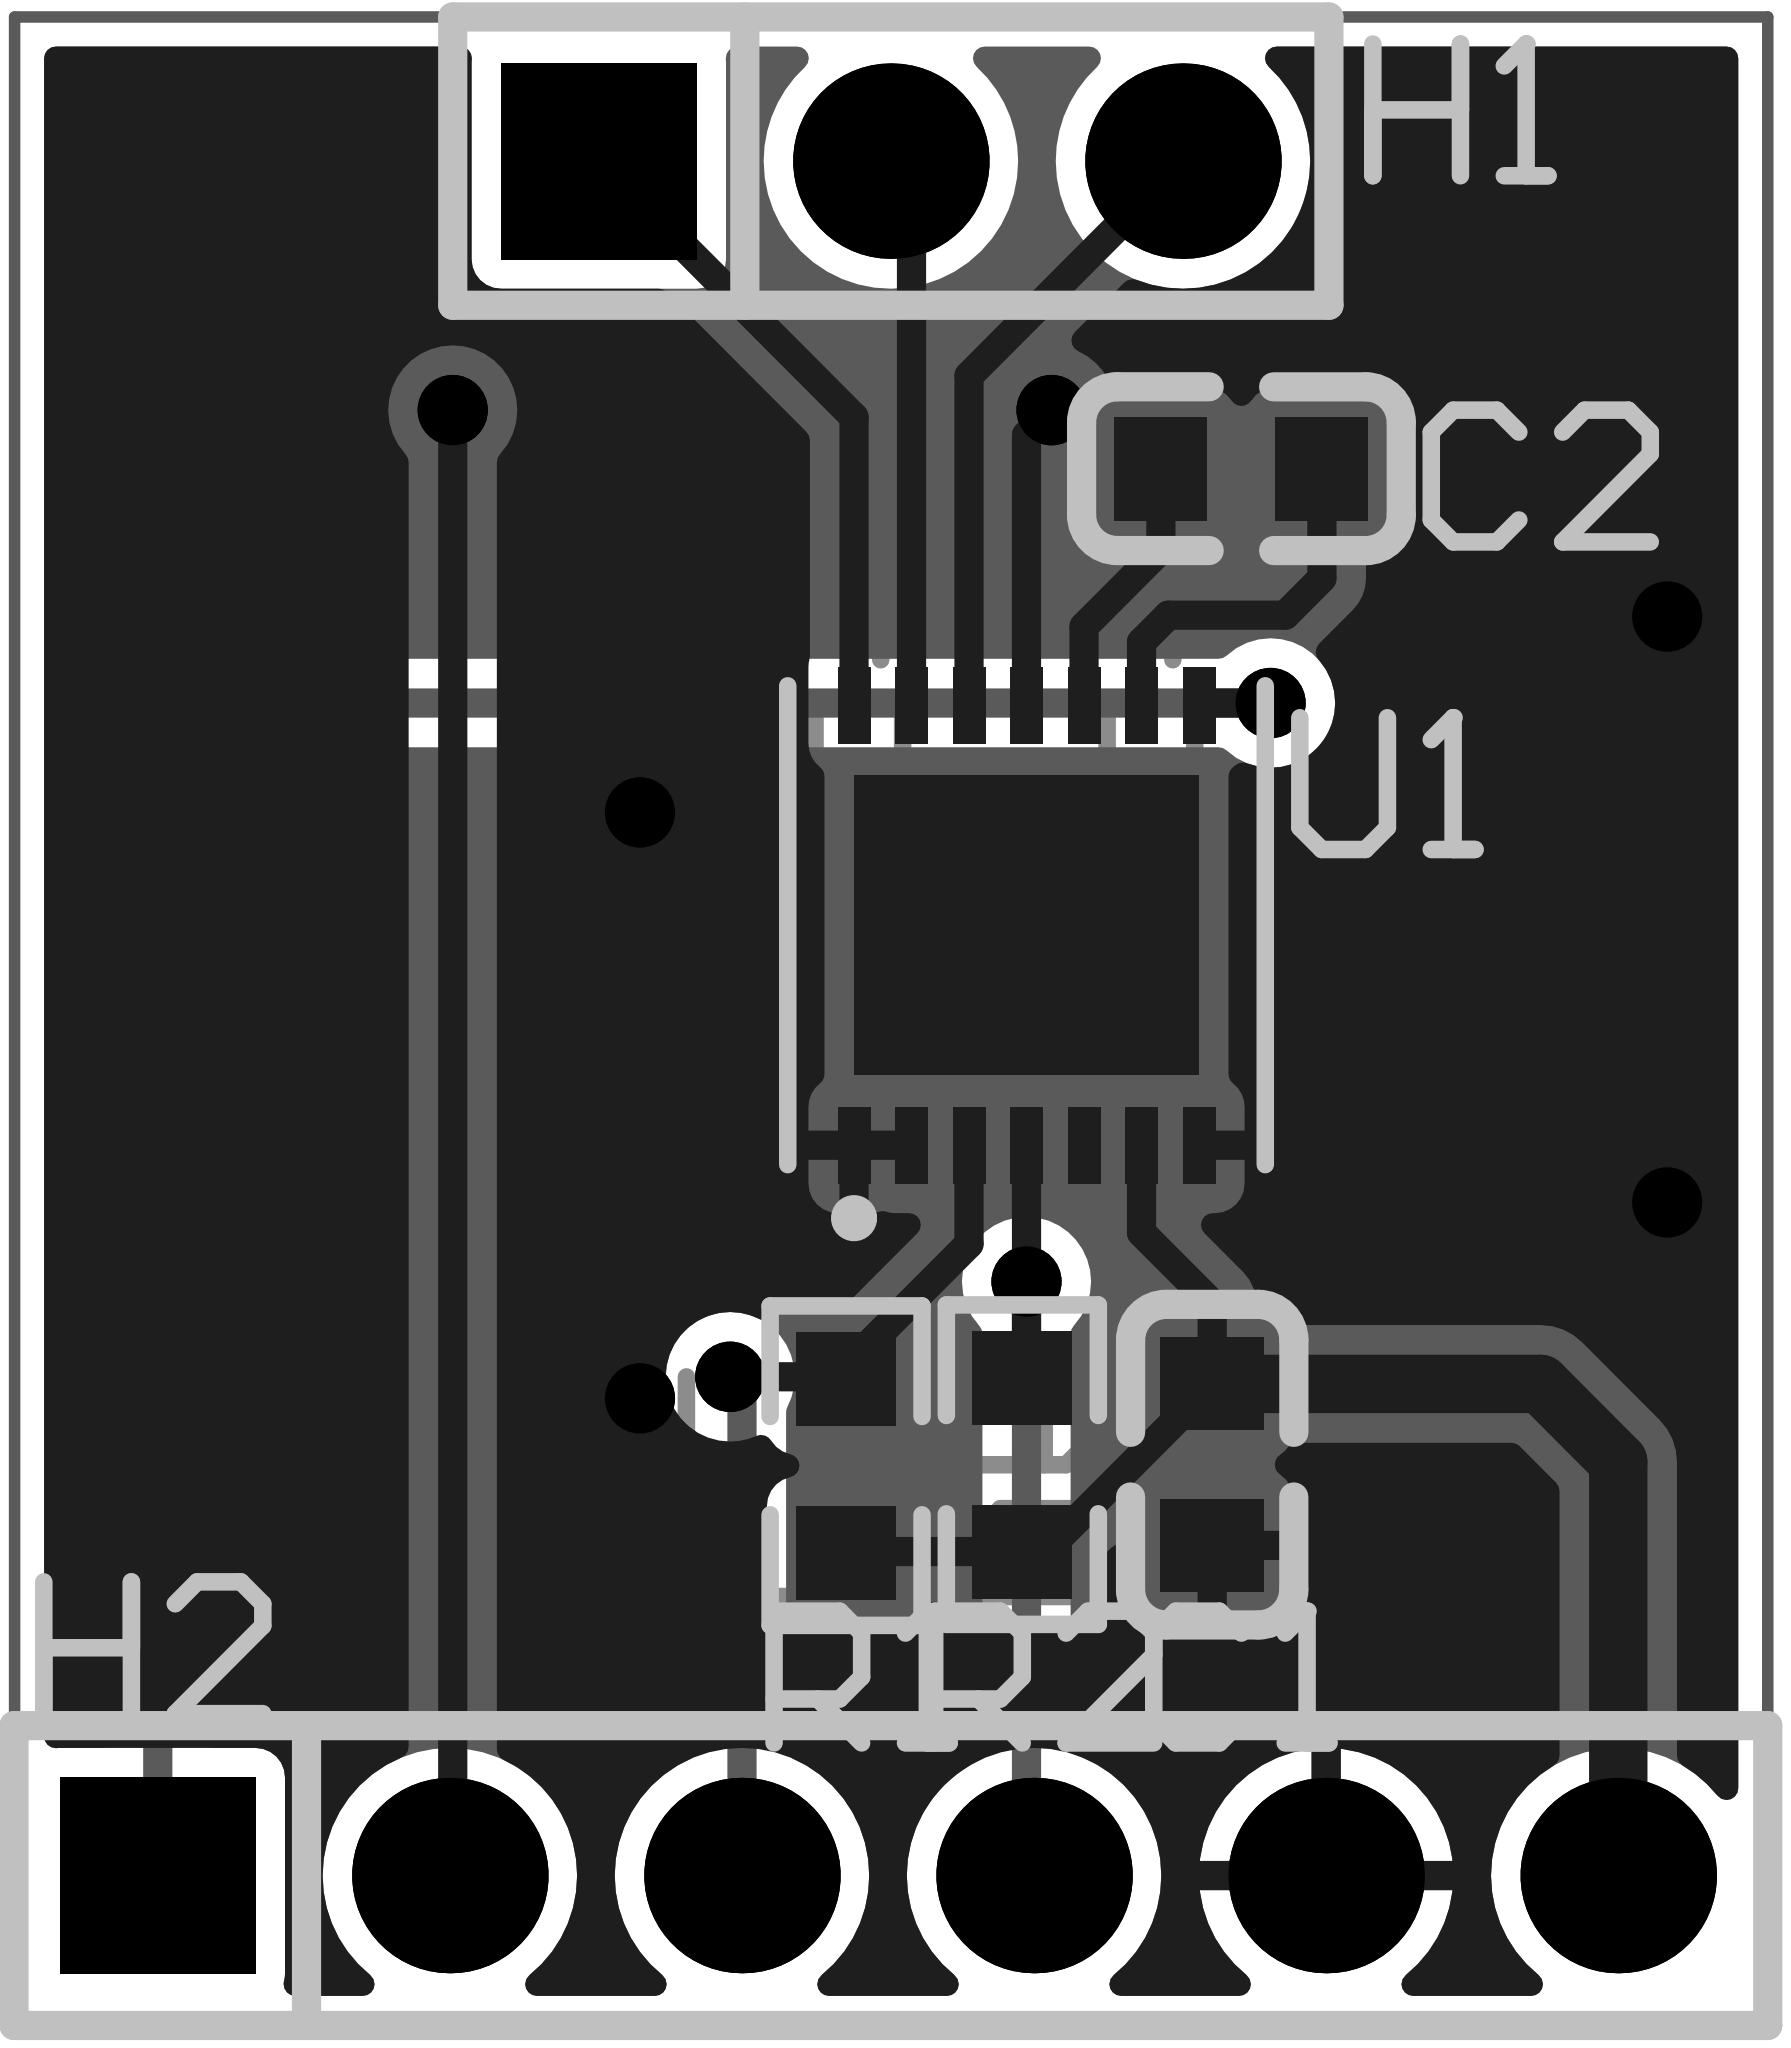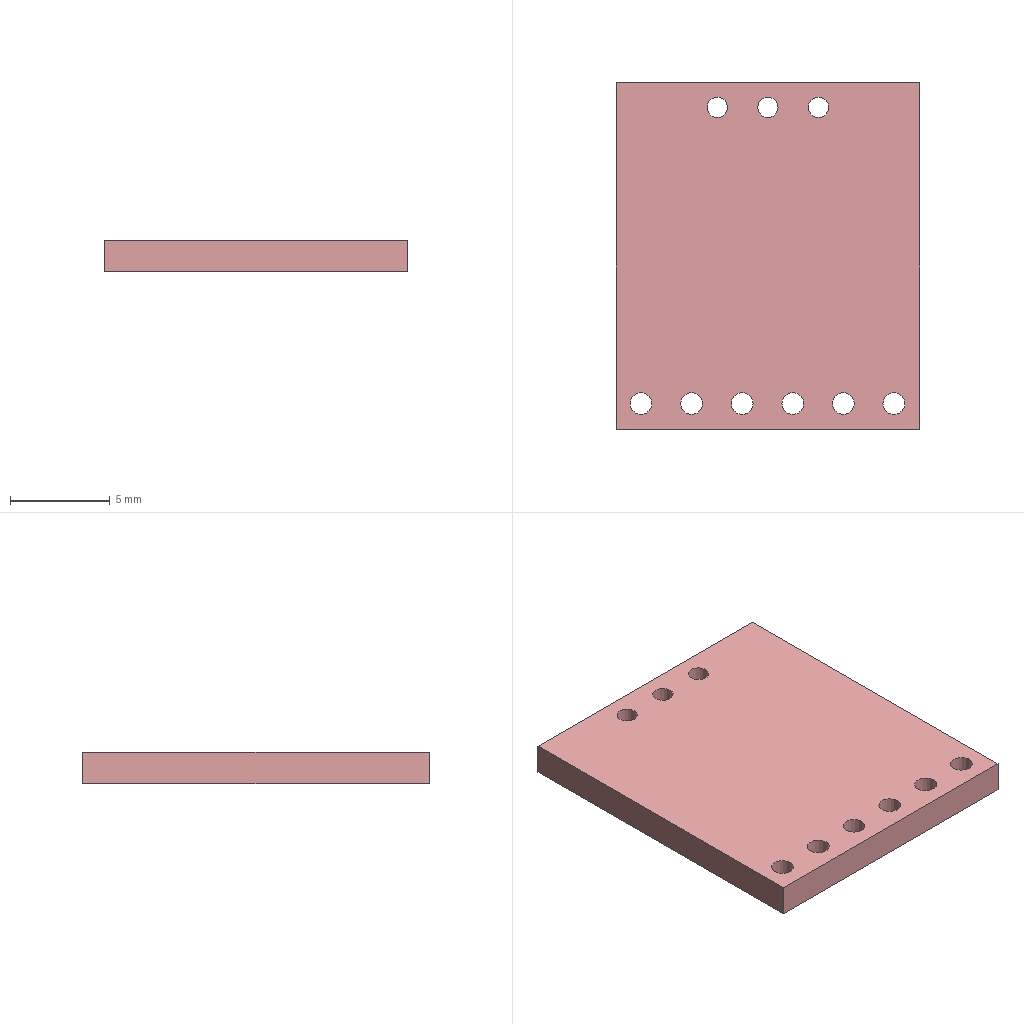Circuit board layout | Altium Designer | box 15.2 x 17.4 x 1.6 mm
Layer stack:
# Altium Designer layer stack of  (unit mm; dielectric type: 0 none, 1 core, 2 prepreg, 3 surface material)
index,name,kind,layer,copper_thickness_mm,dielectric_type,dielectric_thickness_mm,dielectric_material,dielectric_constant
0,Top Paste Mask Layer,other,,,,,,
1,Top Silkscreen Layer,other,,,,,,
2,Top Solder Mask Layer,dielectric,,,3,0.01,,3.3
3,Top Layer,copper,Top Layer,0.035,,,,
4,Dielectric1,dielectric,,,3,1.51,FR4,4.5
5,Bottom Layer,copper,Bottom Layer,0.035,,,,
6,Bottom Solder Mask Layer,dielectric,,,3,0.01,,3.3
7,Bottom Silkscreen Layer,other,,,,,,
8,Bottom Paste Mask Layer,other,,,,,,
# drill layer pairs: low layer,high layer
drill_pair,Top Layer,Bottom Layer
Part placement:
Designator,Comment,Layer,Footprint,Center-X(mm),Center-Y(mm),Rotation
C1,100nF,TopLayer,C0603,88.773,82.55,270
C2,,TopLayer,C0603,89.027,91.186,0
H1,PZ254V-11-03P,TopLayer,HDR-TH_3P-P2.54-V-M_PZ254V-11-03P,85.979,93.853,0
H2,PZ254V-11-06P,TopLayer,HDR-TH_6P-P2.54-V-M,85.954,78.987,0
R1,4.7K,TopLayer,R0603,85.589,82.541,270
R2,4.7K,TopLayer,R0603,87.122,82.55,270
U1,LMP91000SDX/NOPB,TopLayer,WSON-14_L4.0-W4.0-P0.50-BL-EP-1,87.158,87.227,0
Pad and via stacks:
# Altium Designer via and pad stacks of  (unit mm). Each distinct definition once, with the count of objects using it.
# via: kind,start_layer,end_layer,hole_mm,diameter_mm,mode(0 simple;1 top-mid-bottom;2 full stack),diameter_per_layer,count,example_net
# pad: kind,layer,hole_mm,hole_type(0 round;1 square;2 slot),plating,top_size,top_shape(1 round;2 rect;3 octagon;9 rounded rect),mid_size,bottom_size,mode,footprint,size_per_layer,count,example
pad,Top Layer,0,0,plated,0.8x0.9,2,0.8x0.9,0.8x0.9,0,C0603,,4,C1.2
pad,Top Layer,0,0,plated,0.8065x0.864,2,0.8065x0.864,0.8065x0.864,0,R0603,,4,R1.2
pad,Top Layer,0,0,plated,0.28x0.665,2,0.28x0.665,0.28x0.665,0,WSON-14_L4.0-W4.0-P0.50-BL-EP-1,,14,U1.1
pad,Top Layer,0,0,plated,3x2.6,2,3x2.6,3x2.6,0,WSON-14_L4.0-W4.0-P0.50-BL-EP-1,,1,U1.15
pad,Multi-Layer,1.02,0,plated,1.7x1.7,2,1.7x1.7,1.7x1.7,0,HDR-TH_3P-P2.54-V-M_PZ254V-11-03P,,1,H1.1
pad,Multi-Layer,1.02,0,plated,1.7x1.7,1,1.7x1.7,1.7x1.7,0,HDR-TH_3P-P2.54-V-M_PZ254V-11-03P,,2,H1.2
pad,Multi-Layer,1.1,0,plated,1.7x1.7,2,1.7x1.7,1.7x1.7,0,HDR-TH_6P-P2.54-V-M,,1,H2.1
pad,Multi-Layer,1.1,0,plated,1.7x1.7,1,1.7x1.7,1.7x1.7,0,HDR-TH_6P-P2.54-V-M,,5,H2.2
via,Top Layer,Bottom Layer,0.3048,0.61,0,,9,DAC-PH
Copper pours:
name,layer,net,type(0 solid;1 hatched;2 none)
Top Layer-GND,Top Layer,GND,0
Bottom Layer-GND,Bottom Layer,GND,0
Design rules, without the lines most boards share:
# Altium Designer design rules of  (exported by Altium Designer, unit mm)
# columns: name | kind | enabled | priority | scope1 | scope2 | descriptor | typed fields (field=value)
creepage | 65 | enabled | 1 | All | All | Creepage Distance Constraint =(0mil) (All),(All) |